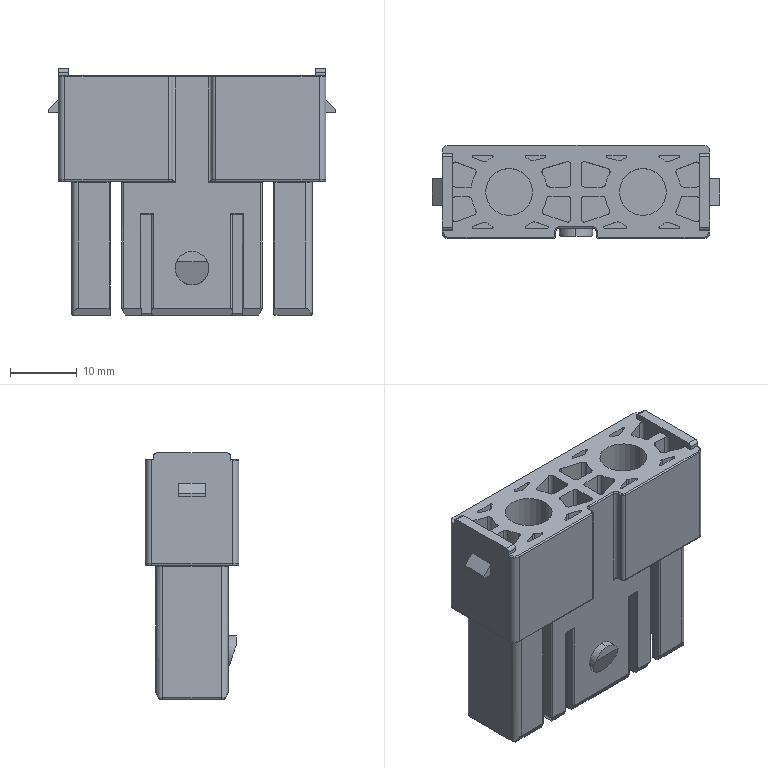Part | NX | features BREP 1 | 1 solid | 385 faces | box 43 x 14 x 36.8 mm | volume 8827 mm3 | cylinder 199 | plane 128 | torus 38 | sphere 14 | spline 6 | commonest cylinder face diameters 0.4 x118 1 x51 11.4 x16 2 x8 7 x4 5 x2